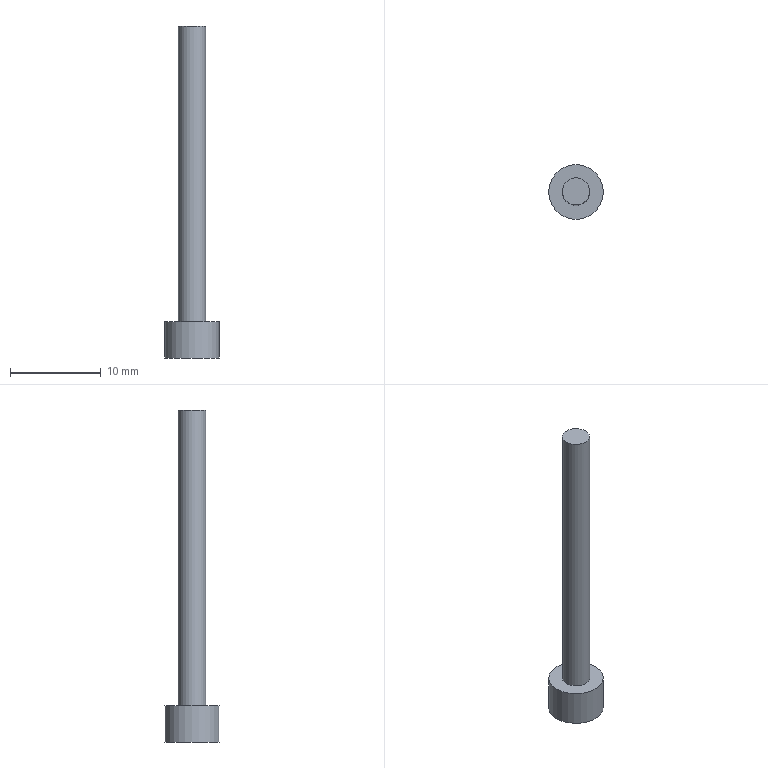Part | STEP file | 1 solid | 5 faces | box 6 x 6 x 36.5 mm | volume 342.826 mm3 | plane 3 | cylinder 2 | commonest cylinder face diameters 3 x1 6 x1
STEP:
#1=CARTESIAN_POINT('',(0.,0.,0.));
#2=DIRECTION('',(0.,0.,1.));
#3=DIRECTION('',(1.,0.,0.));
#4=AXIS2_PLACEMENT_3D('',#1,#2,#3);
#5=CARTESIAN_POINT('',(1484.565,472.48,-48.231));
#6=VERTEX_POINT('',#5);
#7=CARTESIAN_POINT('',(1483.065,472.48,-48.231));
#8=DIRECTION('',(0.,0.,-1.));
#9=DIRECTION('',(1.,0.,0.));
#10=AXIS2_PLACEMENT_3D('',#7,#8,#9);
#11=CIRCLE('',#10,1.5);
#12=CARTESIAN_POINT('',(1483.065,472.48,-48.231));
#13=DIRECTION('',(0.,0.,1.));
#14=DIRECTION('',(-1.,0.,0.));
#15=AXIS2_PLACEMENT_3D('',#12,#13,#14);
#16=PLANE('',#15);
#17=CARTESIAN_POINT('',(-1.5,0.));
#18=CARTESIAN_POINT('',(-1.5,2.598));
#19=CARTESIAN_POINT('',(0.75,1.299));
#20=CARTESIAN_POINT('',(3.,0.));
#21=CARTESIAN_POINT('',(0.75,-1.299));
#22=CARTESIAN_POINT('',(-1.5,-2.598));
#23=CARTESIAN_POINT('',(-1.5,0.));
#24=(BOUNDED_CURVE()B_SPLINE_CURVE(2,(#17,#18,#19,#20,#21,#22,#23),.UNSPECIFIED.,.T.,.F.)B_SPLINE_CURVE_WITH_KNOTS((1,2,2,2,2,1),(-2.094,0.,2.094,4.189,6.283,8.378),.UNSPECIFIED.)CURVE()GEOMETRIC_REPRESENTATION_ITEM()RATIONAL_B_SPLINE_CURVE((1.,0.5,1.,0.5,1.,0.5,1.))REPRESENTATION_ITEM(''));
#25=(GEOMETRIC_REPRESENTATION_CONTEXT(2)PARAMETRIC_REPRESENTATION_CONTEXT()REPRESENTATION_CONTEXT('',''));
#26=DEFINITIONAL_REPRESENTATION('',(#24),#25);
#27=PCURVE('',#16,#26);
#28=CARTESIAN_POINT('',(1483.065,472.48,-80.331));
#29=DIRECTION('',(0.,0.,1.));
#30=DIRECTION('',(-1.,0.,0.));
#31=AXIS2_PLACEMENT_3D('',#28,#29,#30);
#32=CYLINDRICAL_SURFACE('',#31,1.5);
#33=CARTESIAN_POINT('',(9.425,32.1));
#34=DIRECTION('',(-1.,0.));
#35=VECTOR('',#34,1.);
#36=LINE('',#33,#35);
#37=(GEOMETRIC_REPRESENTATION_CONTEXT(2)PARAMETRIC_REPRESENTATION_CONTEXT()REPRESENTATION_CONTEXT('',''));
#38=DEFINITIONAL_REPRESENTATION('',(#36),#37);
#39=PCURVE('',#32,#38);
#40=SURFACE_CURVE('',#11,(#27,#39),.PCURVE_S1.);
#41=EDGE_CURVE('',#6,#6,#40,.T.);
#42=ORIENTED_EDGE('',*,*,#41,.F.);
#43=EDGE_LOOP('',(#42));
#44=FACE_BOUND('',#43,.T.);
#45=ADVANCED_FACE('',(#44),#16,.T.);
#46=ORIENTED_EDGE('',*,*,#41,.T.);
#47=CARTESIAN_POINT('',(1484.565,472.48,-80.731));
#48=VERTEX_POINT('',#47);
#49=CARTESIAN_POINT('',(1484.565,472.48,-80.731));
#50=CARTESIAN_POINT('',(1484.565,472.48,-48.231));
#51=B_SPLINE_CURVE_WITH_KNOTS('',1,(#49,#50),.UNSPECIFIED.,.F.,.F.,(2,2),(-0.4,32.1),.PIECEWISE_BEZIER_KNOTS.);
#52=CARTESIAN_POINT('',(3.142,0.));
#53=DIRECTION('',(0.,1.));
#54=VECTOR('',#53,1.);
#55=LINE('',#52,#54);
#56=(GEOMETRIC_REPRESENTATION_CONTEXT(2)PARAMETRIC_REPRESENTATION_CONTEXT()REPRESENTATION_CONTEXT('',''));
#57=DEFINITIONAL_REPRESENTATION('',(#55),#56);
#58=PCURVE('',#32,#57);
#59=CARTESIAN_POINT('',(9.425,0.));
#60=DIRECTION('',(0.,1.));
#61=VECTOR('',#60,1.);
#62=LINE('',#59,#61);
#63=(GEOMETRIC_REPRESENTATION_CONTEXT(2)PARAMETRIC_REPRESENTATION_CONTEXT()REPRESENTATION_CONTEXT('',''));
#64=DEFINITIONAL_REPRESENTATION('',(#62),#63);
#65=PCURVE('',#32,#64);
#66=SEAM_CURVE('',#51,(#58,#65),.PCURVE_S1.);
#67=EDGE_CURVE('',#48,#6,#66,.T.);
#68=ORIENTED_EDGE('',*,*,#67,.F.);
#69=CARTESIAN_POINT('',(1483.065,472.48,-80.731));
#70=DIRECTION('',(0.,0.,-1.));
#71=DIRECTION('',(1.,0.,0.));
#72=AXIS2_PLACEMENT_3D('',#69,#70,#71);
#73=CIRCLE('',#72,1.5);
#74=CARTESIAN_POINT('',(9.425,-0.4));
#75=DIRECTION('',(-1.,0.));
#76=VECTOR('',#75,1.);
#77=LINE('',#74,#76);
#78=(GEOMETRIC_REPRESENTATION_CONTEXT(2)PARAMETRIC_REPRESENTATION_CONTEXT()REPRESENTATION_CONTEXT('',''));
#79=DEFINITIONAL_REPRESENTATION('',(#77),#78);
#80=PCURVE('',#32,#79);
#81=CARTESIAN_POINT('',(1483.065,472.48,-80.731));
#82=DIRECTION('',(0.,0.,1.));
#83=DIRECTION('',(-1.,0.,0.));
#84=AXIS2_PLACEMENT_3D('',#81,#82,#83);
#85=PLANE('',#84);
#86=CARTESIAN_POINT('',(-1.5,0.));
#87=CARTESIAN_POINT('',(-1.5,2.598));
#88=CARTESIAN_POINT('',(0.75,1.299));
#89=CARTESIAN_POINT('',(3.,0.));
#90=CARTESIAN_POINT('',(0.75,-1.299));
#91=CARTESIAN_POINT('',(-1.5,-2.598));
#92=CARTESIAN_POINT('',(-1.5,0.));
#93=(BOUNDED_CURVE()B_SPLINE_CURVE(2,(#86,#87,#88,#89,#90,#91,#92),.UNSPECIFIED.,.T.,.F.)B_SPLINE_CURVE_WITH_KNOTS((1,2,2,2,2,1),(-2.094,0.,2.094,4.189,6.283,8.378),.UNSPECIFIED.)CURVE()GEOMETRIC_REPRESENTATION_ITEM()RATIONAL_B_SPLINE_CURVE((1.,0.5,1.,0.5,1.,0.5,1.))REPRESENTATION_ITEM(''));
#94=(GEOMETRIC_REPRESENTATION_CONTEXT(2)PARAMETRIC_REPRESENTATION_CONTEXT()REPRESENTATION_CONTEXT('',''));
#95=DEFINITIONAL_REPRESENTATION('',(#93),#94);
#96=PCURVE('',#85,#95);
#97=SURFACE_CURVE('',#73,(#80,#96),.PCURVE_S1.);
#98=EDGE_CURVE('',#48,#48,#97,.T.);
#99=ORIENTED_EDGE('',*,*,#98,.F.);
#100=ORIENTED_EDGE('',*,*,#67,.T.);
#101=EDGE_LOOP('',(#46,#68,#99,#100));
#102=FACE_BOUND('',#101,.T.);
#103=ADVANCED_FACE('',(#102),#32,.T.);
#104=CARTESIAN_POINT('',(1480.065,472.48,-84.731));
#105=VERTEX_POINT('',#104);
#106=CARTESIAN_POINT('',(1483.065,472.48,-84.731));
#107=DIRECTION('',(0.,0.,1.));
#108=DIRECTION('',(-1.,0.,0.));
#109=AXIS2_PLACEMENT_3D('',#106,#107,#108);
#110=CIRCLE('',#109,3.);
#111=CARTESIAN_POINT('',(1483.065,472.48,-84.731));
#112=DIRECTION('',(0.,0.,-1.));
#113=DIRECTION('',(1.,0.,0.));
#114=AXIS2_PLACEMENT_3D('',#111,#112,#113);
#115=PLANE('',#114);
#116=CARTESIAN_POINT('',(-3.,0.));
#117=CARTESIAN_POINT('',(-3.,5.196));
#118=CARTESIAN_POINT('',(1.5,2.598));
#119=CARTESIAN_POINT('',(6.,0.));
#120=CARTESIAN_POINT('',(1.5,-2.598));
#121=CARTESIAN_POINT('',(-3.,-5.196));
#122=CARTESIAN_POINT('',(-3.,0.));
#123=(BOUNDED_CURVE()B_SPLINE_CURVE(2,(#116,#117,#118,#119,#120,#121,#122),.UNSPECIFIED.,.T.,.F.)B_SPLINE_CURVE_WITH_KNOTS((1,2,2,2,2,1),(-2.094,0.,2.094,4.189,6.283,8.378),.UNSPECIFIED.)CURVE()GEOMETRIC_REPRESENTATION_ITEM()RATIONAL_B_SPLINE_CURVE((1.,0.5,1.,0.5,1.,0.5,1.))REPRESENTATION_ITEM(''));
#124=(GEOMETRIC_REPRESENTATION_CONTEXT(2)PARAMETRIC_REPRESENTATION_CONTEXT()REPRESENTATION_CONTEXT('',''));
#125=DEFINITIONAL_REPRESENTATION('',(#123),#124);
#126=PCURVE('',#115,#125);
#127=CARTESIAN_POINT('',(1483.065,472.48,-80.731));
#128=DIRECTION('',(0.,0.,-1.));
#129=DIRECTION('',(-1.,0.,0.));
#130=AXIS2_PLACEMENT_3D('',#127,#128,#129);
#131=CYLINDRICAL_SURFACE('',#130,3.);
#132=CARTESIAN_POINT('',(6.283,4.));
#133=DIRECTION('',(-1.,0.));
#134=VECTOR('',#133,1.);
#135=LINE('',#132,#134);
#136=(GEOMETRIC_REPRESENTATION_CONTEXT(2)PARAMETRIC_REPRESENTATION_CONTEXT()REPRESENTATION_CONTEXT('',''));
#137=DEFINITIONAL_REPRESENTATION('',(#135),#136);
#138=PCURVE('',#131,#137);
#139=SURFACE_CURVE('',#110,(#126,#138),.PCURVE_S1.);
#140=EDGE_CURVE('',#105,#105,#139,.T.);
#141=ORIENTED_EDGE('',*,*,#140,.F.);
#142=EDGE_LOOP('',(#141));
#143=FACE_BOUND('',#142,.T.);
#144=ADVANCED_FACE('',(#143),#115,.T.);
#145=ORIENTED_EDGE('',*,*,#98,.T.);
#146=EDGE_LOOP('',(#145));
#147=FACE_BOUND('',#146,.T.);
#148=CARTESIAN_POINT('',(1486.065,472.48,-80.731));
#149=VERTEX_POINT('',#148);
#150=CARTESIAN_POINT('',(1480.065,472.48,-80.731));
#151=VERTEX_POINT('',#150);
#152=CARTESIAN_POINT('',(1483.065,472.48,-80.731));
#153=DIRECTION('',(0.,0.,-1.));
#154=DIRECTION('',(1.,0.,0.));
#155=AXIS2_PLACEMENT_3D('',#152,#153,#154);
#156=CIRCLE('',#155,3.);
#157=CARTESIAN_POINT('',(-3.,0.));
#158=CARTESIAN_POINT('',(-3.,5.196));
#159=CARTESIAN_POINT('',(1.5,2.598));
#160=CARTESIAN_POINT('',(6.,0.));
#161=CARTESIAN_POINT('',(1.5,-2.598));
#162=CARTESIAN_POINT('',(-3.,-5.196));
#163=CARTESIAN_POINT('',(-3.,0.));
#164=(BOUNDED_CURVE()B_SPLINE_CURVE(2,(#157,#158,#159,#160,#161,#162,#163),.UNSPECIFIED.,.T.,.F.)B_SPLINE_CURVE_WITH_KNOTS((1,2,2,2,2,1),(-2.094,0.,2.094,4.189,6.283,8.378),.UNSPECIFIED.)CURVE()GEOMETRIC_REPRESENTATION_ITEM()RATIONAL_B_SPLINE_CURVE((1.,0.5,1.,0.5,1.,0.5,1.))REPRESENTATION_ITEM(''));
#165=(GEOMETRIC_REPRESENTATION_CONTEXT(2)PARAMETRIC_REPRESENTATION_CONTEXT()REPRESENTATION_CONTEXT('',''));
#166=DEFINITIONAL_REPRESENTATION('',(#164),#165);
#167=PCURVE('',#85,#166);
#168=CARTESIAN_POINT('',(3.142,0.));
#169=DIRECTION('',(1.,0.));
#170=VECTOR('',#169,1.);
#171=LINE('',#168,#170);
#172=(GEOMETRIC_REPRESENTATION_CONTEXT(2)PARAMETRIC_REPRESENTATION_CONTEXT()REPRESENTATION_CONTEXT('',''));
#173=DEFINITIONAL_REPRESENTATION('',(#171),#172);
#174=PCURVE('',#131,#173);
#175=SURFACE_CURVE('',#156,(#167,#174),.PCURVE_S1.);
#176=EDGE_CURVE('',#149,#151,#175,.T.);
#177=ORIENTED_EDGE('',*,*,#176,.F.);
#178=CARTESIAN_POINT('',(1483.065,472.48,-80.731));
#179=DIRECTION('',(0.,0.,-1.));
#180=DIRECTION('',(1.,0.,0.));
#181=AXIS2_PLACEMENT_3D('',#178,#179,#180);
#182=CIRCLE('',#181,3.);
#183=CARTESIAN_POINT('',(-3.,0.));
#184=CARTESIAN_POINT('',(-3.,5.196));
#185=CARTESIAN_POINT('',(1.5,2.598));
#186=CARTESIAN_POINT('',(6.,0.));
#187=CARTESIAN_POINT('',(1.5,-2.598));
#188=CARTESIAN_POINT('',(-3.,-5.196));
#189=CARTESIAN_POINT('',(-3.,0.));
#190=(BOUNDED_CURVE()B_SPLINE_CURVE(2,(#183,#184,#185,#186,#187,#188,#189),.UNSPECIFIED.,.T.,.F.)B_SPLINE_CURVE_WITH_KNOTS((1,2,2,2,2,1),(-2.094,0.,2.094,4.189,6.283,8.378),.UNSPECIFIED.)CURVE()GEOMETRIC_REPRESENTATION_ITEM()RATIONAL_B_SPLINE_CURVE((1.,0.5,1.,0.5,1.,0.5,1.))REPRESENTATION_ITEM(''));
#191=(GEOMETRIC_REPRESENTATION_CONTEXT(2)PARAMETRIC_REPRESENTATION_CONTEXT()REPRESENTATION_CONTEXT('',''));
#192=DEFINITIONAL_REPRESENTATION('',(#190),#191);
#193=PCURVE('',#85,#192);
#194=CARTESIAN_POINT('',(-3.142,0.));
#195=DIRECTION('',(1.,0.));
#196=VECTOR('',#195,1.);
#197=LINE('',#194,#196);
#198=(GEOMETRIC_REPRESENTATION_CONTEXT(2)PARAMETRIC_REPRESENTATION_CONTEXT()REPRESENTATION_CONTEXT('',''));
#199=DEFINITIONAL_REPRESENTATION('',(#197),#198);
#200=PCURVE('',#131,#199);
#201=SURFACE_CURVE('',#182,(#193,#200),.PCURVE_S1.);
#202=EDGE_CURVE('',#151,#149,#201,.T.);
#203=ORIENTED_EDGE('',*,*,#202,.F.);
#204=EDGE_LOOP('',(#177,#203));
#205=FACE_BOUND('',#204,.T.);
#206=ADVANCED_FACE('',(#147,#205),#85,.T.);
#207=ORIENTED_EDGE('',*,*,#140,.T.);
#208=CARTESIAN_POINT('',(1480.065,472.48,-80.731));
#209=CARTESIAN_POINT('',(1480.065,472.48,-84.731));
#210=B_SPLINE_CURVE_WITH_KNOTS('',1,(#208,#209),.UNSPECIFIED.,.F.,.F.,(2,2),(0.,4.),.PIECEWISE_BEZIER_KNOTS.);
#211=CARTESIAN_POINT('',(0.,0.));
#212=DIRECTION('',(0.,1.));
#213=VECTOR('',#212,1.);
#214=LINE('',#211,#213);
#215=(GEOMETRIC_REPRESENTATION_CONTEXT(2)PARAMETRIC_REPRESENTATION_CONTEXT()REPRESENTATION_CONTEXT('',''));
#216=DEFINITIONAL_REPRESENTATION('',(#214),#215);
#217=PCURVE('',#131,#216);
#218=CARTESIAN_POINT('',(6.283,0.));
#219=DIRECTION('',(0.,1.));
#220=VECTOR('',#219,1.);
#221=LINE('',#218,#220);
#222=(GEOMETRIC_REPRESENTATION_CONTEXT(2)PARAMETRIC_REPRESENTATION_CONTEXT()REPRESENTATION_CONTEXT('',''));
#223=DEFINITIONAL_REPRESENTATION('',(#221),#222);
#224=PCURVE('',#131,#223);
#225=SEAM_CURVE('',#210,(#217,#224),.PCURVE_S1.);
#226=EDGE_CURVE('',#151,#105,#225,.T.);
#227=ORIENTED_EDGE('',*,*,#226,.F.);
#228=ORIENTED_EDGE('',*,*,#202,.T.);
#229=ORIENTED_EDGE('',*,*,#176,.T.);
#230=ORIENTED_EDGE('',*,*,#226,.T.);
#231=EDGE_LOOP('',(#207,#227,#228,#229,#230));
#232=FACE_BOUND('',#231,.T.);
#233=ADVANCED_FACE('',(#232),#131,.T.);
#234=CLOSED_SHELL('',(#45,#103,#144,#206,#233));
#235=MANIFOLD_SOLID_BREP('',#234);
#236=(LENGTH_UNIT()NAMED_UNIT(*)SI_UNIT(.MILLI.,.METRE.));
#237=UNCERTAINTY_MEASURE_WITH_UNIT(LENGTH_MEASURE(0.000005),#236,'','');
#238=(NAMED_UNIT(*)PLANE_ANGLE_UNIT()SI_UNIT($,.RADIAN.));
#239=(NAMED_UNIT(*)SI_UNIT($,.STERADIAN.)SOLID_ANGLE_UNIT());
#240=(GEOMETRIC_REPRESENTATION_CONTEXT(3)GLOBAL_UNCERTAINTY_ASSIGNED_CONTEXT((#237))GLOBAL_UNIT_ASSIGNED_CONTEXT((#236,#238,#239))REPRESENTATION_CONTEXT('',''));
#241=ADVANCED_BREP_SHAPE_REPRESENTATION('',(#4,#235),#240);